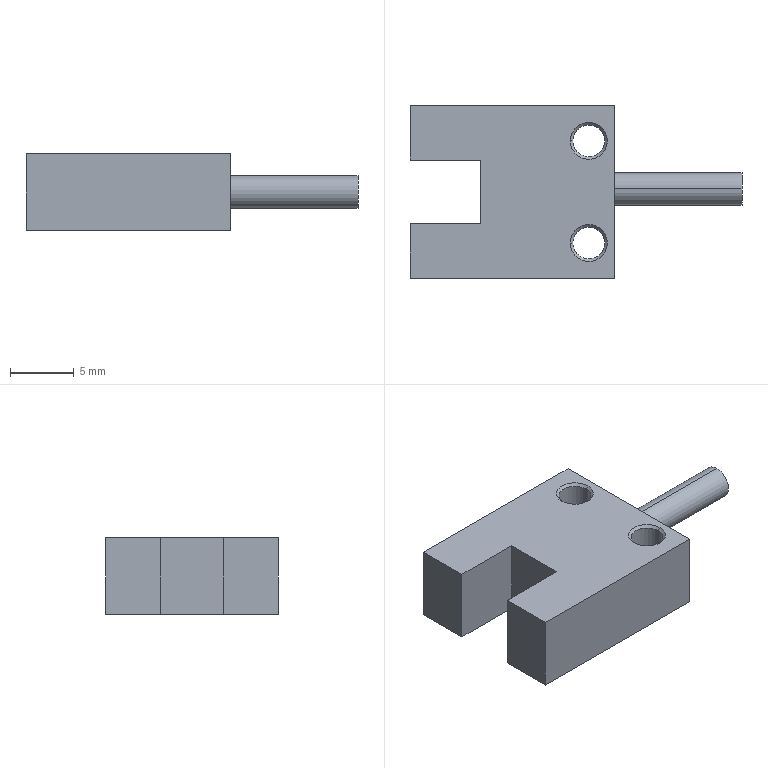Part | SolidWorks | features BaseBody 1 | 1 solid | 25 faces | box 26 x 13.5 x 6 mm | volume 1123 mm3 | plane 11 | cone 8 | cylinder 6 | commonest cylinder face diameters 2.5 x4 2.557 x2
STEP:
#1=CARTESIAN_POINT('',(4.191,-0.7465,0.2));
#2=VERTEX_POINT('',#1);
#3=CARTESIAN_POINT('',(1.691,-0.7465,0.2));
#4=VERTEX_POINT('',#3);
#5=CARTESIAN_POINT('',(2.941,-0.7465,0.2));
#6=DIRECTION('',(0.,0.,-1.));
#7=DIRECTION('',(-1.,0.,0.));
#8=AXIS2_PLACEMENT_3D('',#5,#6,#7);
#9=CIRCLE('',#8,1.25);
#10=EDGE_CURVE('',#2,#4,#9,.T.);
#11=ORIENTED_EDGE('',*,*,#10,.F.);
#12=CARTESIAN_POINT('',(4.391,-0.7465,0.));
#13=VERTEX_POINT('',#12);
#14=CARTESIAN_POINT('',(4.391,-0.7465,0.));
#15=DIRECTION('',(0.7071,0.,-0.7071));
#16=VECTOR('',#15,1000.);
#17=LINE('',#14,#16);
#18=EDGE_CURVE('',#2,#13,#17,.T.);
#19=ORIENTED_EDGE('',*,*,#18,.T.);
#20=CARTESIAN_POINT('',(1.491,-0.7465,0.));
#21=VERTEX_POINT('',#20);
#22=CARTESIAN_POINT('',(2.941,-0.7465,0.));
#23=DIRECTION('',(0.,0.,-1.));
#24=DIRECTION('',(-1.,0.,0.));
#25=AXIS2_PLACEMENT_3D('',#22,#23,#24);
#26=CIRCLE('',#25,1.45);
#27=EDGE_CURVE('',#13,#21,#26,.T.);
#28=ORIENTED_EDGE('',*,*,#27,.T.);
#29=CARTESIAN_POINT('',(1.491,-0.7465,0.));
#30=DIRECTION('',(-0.7071,0.,-0.7071));
#31=VECTOR('',#30,1000.);
#32=LINE('',#29,#31);
#33=EDGE_CURVE('',#4,#21,#32,.T.);
#34=ORIENTED_EDGE('',*,*,#33,.F.);
#35=EDGE_LOOP('',(#11,#19,#28,#34));
#36=FACE_OUTER_BOUND('',#35,.T.);
#37=CARTESIAN_POINT('',(2.941,-0.7465,0.));
#38=DIRECTION('',(0.,0.,-1.));
#39=DIRECTION('',(-1.,0.,0.));
#40=AXIS2_PLACEMENT_3D('',#37,#38,#39);
#41=CONICAL_SURFACE('',#40,1.45,0.7854);
#42=ADVANCED_FACE('',(#36),#41,.F.);
#43=CARTESIAN_POINT('',(4.191,7.253,0.2));
#44=VERTEX_POINT('',#43);
#45=CARTESIAN_POINT('',(1.691,7.253,0.2));
#46=VERTEX_POINT('',#45);
#47=CARTESIAN_POINT('',(2.941,7.253,0.2));
#48=DIRECTION('',(0.,0.,-1.));
#49=DIRECTION('',(-1.,0.,0.));
#50=AXIS2_PLACEMENT_3D('',#47,#48,#49);
#51=CIRCLE('',#50,1.25);
#52=EDGE_CURVE('',#44,#46,#51,.T.);
#53=ORIENTED_EDGE('',*,*,#52,.F.);
#54=CARTESIAN_POINT('',(4.391,7.253,0.));
#55=VERTEX_POINT('',#54);
#56=CARTESIAN_POINT('',(4.391,7.253,0.));
#57=DIRECTION('',(0.7071,0.,-0.7071));
#58=VECTOR('',#57,1000.);
#59=LINE('',#56,#58);
#60=EDGE_CURVE('',#44,#55,#59,.T.);
#61=ORIENTED_EDGE('',*,*,#60,.T.);
#62=CARTESIAN_POINT('',(1.491,7.253,0.));
#63=VERTEX_POINT('',#62);
#64=CARTESIAN_POINT('',(2.941,7.253,0.));
#65=DIRECTION('',(0.,0.,-1.));
#66=DIRECTION('',(-1.,0.,0.));
#67=AXIS2_PLACEMENT_3D('',#64,#65,#66);
#68=CIRCLE('',#67,1.45);
#69=EDGE_CURVE('',#55,#63,#68,.T.);
#70=ORIENTED_EDGE('',*,*,#69,.T.);
#71=CARTESIAN_POINT('',(1.491,7.253,0.));
#72=DIRECTION('',(-0.7071,0.,-0.7071));
#73=VECTOR('',#72,1000.);
#74=LINE('',#71,#73);
#75=EDGE_CURVE('',#46,#63,#74,.T.);
#76=ORIENTED_EDGE('',*,*,#75,.F.);
#77=EDGE_LOOP('',(#53,#61,#70,#76));
#78=FACE_OUTER_BOUND('',#77,.T.);
#79=CARTESIAN_POINT('',(2.941,7.253,0.));
#80=DIRECTION('',(0.,0.,-1.));
#81=DIRECTION('',(-1.,0.,0.));
#82=AXIS2_PLACEMENT_3D('',#79,#80,#81);
#83=CONICAL_SURFACE('',#82,1.45,0.7854);
#84=ADVANCED_FACE('',(#78),#83,.F.);
#85=CARTESIAN_POINT('',(4.191,-0.7465,5.8));
#86=VERTEX_POINT('',#85);
#87=CARTESIAN_POINT('',(1.691,-0.7465,5.8));
#88=VERTEX_POINT('',#87);
#89=CARTESIAN_POINT('',(2.941,-0.7465,5.8));
#90=DIRECTION('',(0.,0.,-1.));
#91=DIRECTION('',(-1.,0.,0.));
#92=AXIS2_PLACEMENT_3D('',#89,#90,#91);
#93=CIRCLE('',#92,1.25);
#94=EDGE_CURVE('',#86,#88,#93,.T.);
#95=ORIENTED_EDGE('',*,*,#94,.F.);
#96=CARTESIAN_POINT('',(4.191,-0.7465,6.));
#97=DIRECTION('',(0.,0.,-1.));
#98=VECTOR('',#97,1000.);
#99=LINE('',#96,#98);
#100=EDGE_CURVE('',#86,#2,#99,.T.);
#101=ORIENTED_EDGE('',*,*,#100,.T.);
#102=ORIENTED_EDGE('',*,*,#10,.T.);
#103=CARTESIAN_POINT('',(1.691,-0.7465,6.));
#104=DIRECTION('',(0.,0.,-1.));
#105=VECTOR('',#104,1000.);
#106=LINE('',#103,#105);
#107=EDGE_CURVE('',#88,#4,#106,.T.);
#108=ORIENTED_EDGE('',*,*,#107,.F.);
#109=EDGE_LOOP('',(#95,#101,#102,#108));
#110=FACE_OUTER_BOUND('',#109,.T.);
#111=CARTESIAN_POINT('',(2.941,-0.7465,6.));
#112=DIRECTION('',(0.,0.,-1.));
#113=DIRECTION('',(-1.,0.,0.));
#114=AXIS2_PLACEMENT_3D('',#111,#112,#113);
#115=CYLINDRICAL_SURFACE('',#114,1.25);
#116=ADVANCED_FACE('',(#110),#115,.F.);
#117=CARTESIAN_POINT('',(4.191,7.253,5.8));
#118=VERTEX_POINT('',#117);
#119=CARTESIAN_POINT('',(1.691,7.253,5.8));
#120=VERTEX_POINT('',#119);
#121=CARTESIAN_POINT('',(2.941,7.253,5.8));
#122=DIRECTION('',(0.,0.,-1.));
#123=DIRECTION('',(-1.,0.,0.));
#124=AXIS2_PLACEMENT_3D('',#121,#122,#123);
#125=CIRCLE('',#124,1.25);
#126=EDGE_CURVE('',#118,#120,#125,.T.);
#127=ORIENTED_EDGE('',*,*,#126,.F.);
#128=CARTESIAN_POINT('',(4.191,7.253,6.));
#129=DIRECTION('',(0.,0.,-1.));
#130=VECTOR('',#129,1000.);
#131=LINE('',#128,#130);
#132=EDGE_CURVE('',#118,#44,#131,.T.);
#133=ORIENTED_EDGE('',*,*,#132,.T.);
#134=ORIENTED_EDGE('',*,*,#52,.T.);
#135=CARTESIAN_POINT('',(1.691,7.253,6.));
#136=DIRECTION('',(0.,0.,-1.));
#137=VECTOR('',#136,1000.);
#138=LINE('',#135,#137);
#139=EDGE_CURVE('',#120,#46,#138,.T.);
#140=ORIENTED_EDGE('',*,*,#139,.F.);
#141=EDGE_LOOP('',(#127,#133,#134,#140));
#142=FACE_OUTER_BOUND('',#141,.T.);
#143=CARTESIAN_POINT('',(2.941,7.253,6.));
#144=DIRECTION('',(0.,0.,-1.));
#145=DIRECTION('',(-1.,0.,0.));
#146=AXIS2_PLACEMENT_3D('',#143,#144,#145);
#147=CYLINDRICAL_SURFACE('',#146,1.25);
#148=ADVANCED_FACE('',(#142),#147,.F.);
#149=CARTESIAN_POINT('',(4.941,3.503,4.278));
#150=VERTEX_POINT('',#149);
#151=CARTESIAN_POINT('',(4.941,3.503,1.722));
#152=VERTEX_POINT('',#151);
#153=CARTESIAN_POINT('',(4.941,3.503,3.));
#154=DIRECTION('',(-1.,0.,0.));
#155=DIRECTION('',(0.,0.,-1.));
#156=AXIS2_PLACEMENT_3D('',#153,#154,#155);
#157=CIRCLE('',#156,1.278);
#158=EDGE_CURVE('',#150,#152,#157,.T.);
#159=ORIENTED_EDGE('',*,*,#158,.F.);
#160=CARTESIAN_POINT('',(14.941,3.503,4.278));
#161=VERTEX_POINT('',#160);
#162=CARTESIAN_POINT('',(4.941,3.503,4.278));
#163=DIRECTION('',(1.,0.,0.));
#164=VECTOR('',#163,1000.);
#165=LINE('',#162,#164);
#166=EDGE_CURVE('',#150,#161,#165,.T.);
#167=ORIENTED_EDGE('',*,*,#166,.T.);
#168=CARTESIAN_POINT('',(14.941,3.503,1.722));
#169=VERTEX_POINT('',#168);
#170=CARTESIAN_POINT('',(14.941,3.503,3.));
#171=DIRECTION('',(-1.,0.,0.));
#172=DIRECTION('',(0.,0.,-1.));
#173=AXIS2_PLACEMENT_3D('',#170,#171,#172);
#174=CIRCLE('',#173,1.278);
#175=EDGE_CURVE('',#161,#169,#174,.T.);
#176=ORIENTED_EDGE('',*,*,#175,.T.);
#177=CARTESIAN_POINT('',(4.941,3.503,1.722));
#178=DIRECTION('',(1.,0.,0.));
#179=VECTOR('',#178,1000.);
#180=LINE('',#177,#179);
#181=EDGE_CURVE('',#152,#169,#180,.T.);
#182=ORIENTED_EDGE('',*,*,#181,.F.);
#183=EDGE_LOOP('',(#159,#167,#176,#182));
#184=FACE_OUTER_BOUND('',#183,.T.);
#185=CARTESIAN_POINT('',(4.941,3.503,3.));
#186=DIRECTION('',(1.,0.,0.));
#187=DIRECTION('',(0.,0.,-1.));
#188=AXIS2_PLACEMENT_3D('',#185,#186,#187);
#189=CYLINDRICAL_SURFACE('',#188,1.278);
#190=ADVANCED_FACE('',(#184),#189,.T.);
#191=ORIENTED_EDGE('',*,*,#94,.T.);
#192=CARTESIAN_POINT('',(1.491,-0.7465,6.));
#193=VERTEX_POINT('',#192);
#194=CARTESIAN_POINT('',(1.491,-0.7465,6.));
#195=DIRECTION('',(-0.7071,0.,0.7071));
#196=VECTOR('',#195,1000.);
#197=LINE('',#194,#196);
#198=EDGE_CURVE('',#88,#193,#197,.T.);
#199=ORIENTED_EDGE('',*,*,#198,.T.);
#200=CARTESIAN_POINT('',(4.391,-0.7465,6.));
#201=VERTEX_POINT('',#200);
#202=CARTESIAN_POINT('',(2.941,-0.7465,6.));
#203=DIRECTION('',(0.,0.,-1.));
#204=DIRECTION('',(1.,0.,0.));
#205=AXIS2_PLACEMENT_3D('',#202,#203,#204);
#206=CIRCLE('',#205,1.45);
#207=EDGE_CURVE('',#201,#193,#206,.T.);
#208=ORIENTED_EDGE('',*,*,#207,.F.);
#209=CARTESIAN_POINT('',(4.391,-0.7465,6.));
#210=DIRECTION('',(0.7071,0.,0.7071));
#211=VECTOR('',#210,1000.);
#212=LINE('',#209,#211);
#213=EDGE_CURVE('',#86,#201,#212,.T.);
#214=ORIENTED_EDGE('',*,*,#213,.F.);
#215=EDGE_LOOP('',(#191,#199,#208,#214));
#216=FACE_OUTER_BOUND('',#215,.T.);
#217=CARTESIAN_POINT('',(2.941,-0.7465,6.));
#218=DIRECTION('',(0.,0.,1.));
#219=DIRECTION('',(1.,0.,0.));
#220=AXIS2_PLACEMENT_3D('',#217,#218,#219);
#221=CONICAL_SURFACE('',#220,1.45,0.7854);
#222=ADVANCED_FACE('',(#216),#221,.F.);
#223=ORIENTED_EDGE('',*,*,#126,.T.);
#224=CARTESIAN_POINT('',(1.491,7.253,6.));
#225=VERTEX_POINT('',#224);
#226=CARTESIAN_POINT('',(1.491,7.253,6.));
#227=DIRECTION('',(-0.7071,0.,0.7071));
#228=VECTOR('',#227,1000.);
#229=LINE('',#226,#228);
#230=EDGE_CURVE('',#120,#225,#229,.T.);
#231=ORIENTED_EDGE('',*,*,#230,.T.);
#232=CARTESIAN_POINT('',(4.391,7.253,6.));
#233=VERTEX_POINT('',#232);
#234=CARTESIAN_POINT('',(2.941,7.253,6.));
#235=DIRECTION('',(0.,0.,-1.));
#236=DIRECTION('',(1.,0.,0.));
#237=AXIS2_PLACEMENT_3D('',#234,#235,#236);
#238=CIRCLE('',#237,1.45);
#239=EDGE_CURVE('',#233,#225,#238,.T.);
#240=ORIENTED_EDGE('',*,*,#239,.F.);
#241=CARTESIAN_POINT('',(4.391,7.253,6.));
#242=DIRECTION('',(0.7071,0.,0.7071));
#243=VECTOR('',#242,1000.);
#244=LINE('',#241,#243);
#245=EDGE_CURVE('',#118,#233,#244,.T.);
#246=ORIENTED_EDGE('',*,*,#245,.F.);
#247=EDGE_LOOP('',(#223,#231,#240,#246));
#248=FACE_OUTER_BOUND('',#247,.T.);
#249=CARTESIAN_POINT('',(2.941,7.253,6.));
#250=DIRECTION('',(0.,0.,1.));
#251=DIRECTION('',(1.,0.,0.));
#252=AXIS2_PLACEMENT_3D('',#249,#250,#251);
#253=CONICAL_SURFACE('',#252,1.45,0.7854);
#254=ADVANCED_FACE('',(#248),#253,.F.);
#255=CARTESIAN_POINT('',(2.941,-0.7465,0.));
#256=DIRECTION('',(0.,0.,-1.));
#257=DIRECTION('',(-1.,0.,0.));
#258=AXIS2_PLACEMENT_3D('',#255,#256,#257);
#259=CIRCLE('',#258,1.45);
#260=EDGE_CURVE('',#21,#13,#259,.T.);
#261=ORIENTED_EDGE('',*,*,#260,.F.);
#262=ORIENTED_EDGE('',*,*,#27,.F.);
#263=EDGE_LOOP('',(#261,#262));
#264=FACE_BOUND('',#263,.T.);
#265=CARTESIAN_POINT('',(2.941,7.253,0.));
#266=DIRECTION('',(0.,0.,-1.));
#267=DIRECTION('',(-1.,0.,0.));
#268=AXIS2_PLACEMENT_3D('',#265,#266,#267);
#269=CIRCLE('',#268,1.45);
#270=EDGE_CURVE('',#63,#55,#269,.T.);
#271=ORIENTED_EDGE('',*,*,#270,.F.);
#272=ORIENTED_EDGE('',*,*,#69,.F.);
#273=EDGE_LOOP('',(#271,#272));
#274=FACE_BOUND('',#273,.T.);
#275=CARTESIAN_POINT('',(-11.059,0.7535,0.));
#276=VERTEX_POINT('',#275);
#277=CARTESIAN_POINT('',(-11.059,-3.497,0.));
#278=VERTEX_POINT('',#277);
#279=CARTESIAN_POINT('',(-11.059,3.253,0.));
#280=DIRECTION('',(0.,-1.,0.));
#281=VECTOR('',#280,1000.);
#282=LINE('',#279,#281);
#283=EDGE_CURVE('',#276,#278,#282,.T.);
#284=ORIENTED_EDGE('',*,*,#283,.F.);
#285=CARTESIAN_POINT('',(-5.559,0.7535,0.));
#286=VERTEX_POINT('',#285);
#287=CARTESIAN_POINT('',(-3.491,0.7535,0.));
#288=DIRECTION('',(-1.,0.,0.));
#289=VECTOR('',#288,1000.);
#290=LINE('',#287,#289);
#291=EDGE_CURVE('',#286,#276,#290,.T.);
#292=ORIENTED_EDGE('',*,*,#291,.F.);
#293=CARTESIAN_POINT('',(-5.559,5.753,0.));
#294=VERTEX_POINT('',#293);
#295=CARTESIAN_POINT('',(-5.559,3.253,0.));
#296=DIRECTION('',(0.,-1.,0.));
#297=VECTOR('',#296,1000.);
#298=LINE('',#295,#297);
#299=EDGE_CURVE('',#294,#286,#298,.T.);
#300=ORIENTED_EDGE('',*,*,#299,.F.);
#301=CARTESIAN_POINT('',(-11.059,5.753,0.));
#302=VERTEX_POINT('',#301);
#303=CARTESIAN_POINT('',(-3.491,5.753,0.));
#304=DIRECTION('',(1.,0.,0.));
#305=VECTOR('',#304,1000.);
#306=LINE('',#303,#305);
#307=EDGE_CURVE('',#302,#294,#306,.T.);
#308=ORIENTED_EDGE('',*,*,#307,.F.);
#309=CARTESIAN_POINT('',(-11.059,10.003,0.));
#310=VERTEX_POINT('',#309);
#311=CARTESIAN_POINT('',(-11.059,3.253,0.));
#312=DIRECTION('',(0.,-1.,0.));
#313=VECTOR('',#312,1000.);
#314=LINE('',#311,#313);
#315=EDGE_CURVE('',#310,#302,#314,.T.);
#316=ORIENTED_EDGE('',*,*,#315,.F.);
#317=CARTESIAN_POINT('',(4.941,10.003,0.));
#318=VERTEX_POINT('',#317);
#319=CARTESIAN_POINT('',(-3.491,10.003,0.));
#320=DIRECTION('',(-1.,0.,0.));
#321=VECTOR('',#320,1000.);
#322=LINE('',#319,#321);
#323=EDGE_CURVE('',#318,#310,#322,.T.);
#324=ORIENTED_EDGE('',*,*,#323,.F.);
#325=CARTESIAN_POINT('',(4.941,-3.497,0.));
#326=VERTEX_POINT('',#325);
#327=CARTESIAN_POINT('',(4.941,3.253,0.));
#328=DIRECTION('',(0.,1.,0.));
#329=VECTOR('',#328,1000.);
#330=LINE('',#327,#329);
#331=EDGE_CURVE('',#326,#318,#330,.T.);
#332=ORIENTED_EDGE('',*,*,#331,.F.);
#333=CARTESIAN_POINT('',(-3.491,-3.497,0.));
#334=DIRECTION('',(1.,0.,0.));
#335=VECTOR('',#334,1000.);
#336=LINE('',#333,#335);
#337=EDGE_CURVE('',#278,#326,#336,.T.);
#338=ORIENTED_EDGE('',*,*,#337,.F.);
#339=EDGE_LOOP('',(#284,#292,#300,#308,#316,#324,#332,#338));
#340=FACE_OUTER_BOUND('',#339,.T.);
#341=CARTESIAN_POINT('',(-3.491,3.253,0.));
#342=DIRECTION('',(0.,0.,1.));
#343=DIRECTION('',(1.,0.,0.));
#344=AXIS2_PLACEMENT_3D('',#341,#342,#343);
#345=PLANE('',#344);
#346=ADVANCED_FACE('',(#264,#274,#340),#345,.F.);
#347=ORIENTED_EDGE('',*,*,#18,.F.);
#348=CARTESIAN_POINT('',(2.941,-0.7465,0.2));
#349=DIRECTION('',(0.,0.,-1.));
#350=DIRECTION('',(-1.,0.,0.));
#351=AXIS2_PLACEMENT_3D('',#348,#349,#350);
#352=CIRCLE('',#351,1.25);
#353=EDGE_CURVE('',#4,#2,#352,.T.);
#354=ORIENTED_EDGE('',*,*,#353,.F.);
#355=ORIENTED_EDGE('',*,*,#33,.T.);
#356=ORIENTED_EDGE('',*,*,#260,.T.);
#357=EDGE_LOOP('',(#347,#354,#355,#356));
#358=FACE_OUTER_BOUND('',#357,.T.);
#359=CARTESIAN_POINT('',(2.941,-0.7465,0.));
#360=DIRECTION('',(0.,0.,-1.));
#361=DIRECTION('',(-1.,0.,0.));
#362=AXIS2_PLACEMENT_3D('',#359,#360,#361);
#363=CONICAL_SURFACE('',#362,1.45,0.7854);
#364=ADVANCED_FACE('',(#358),#363,.F.);
#365=ORIENTED_EDGE('',*,*,#60,.F.);
#366=CARTESIAN_POINT('',(2.941,7.253,0.2));
#367=DIRECTION('',(0.,0.,-1.));
#368=DIRECTION('',(-1.,0.,0.));
#369=AXIS2_PLACEMENT_3D('',#366,#367,#368);
#370=CIRCLE('',#369,1.25);
#371=EDGE_CURVE('',#46,#44,#370,.T.);
#372=ORIENTED_EDGE('',*,*,#371,.F.);
#373=ORIENTED_EDGE('',*,*,#75,.T.);
#374=ORIENTED_EDGE('',*,*,#270,.T.);
#375=EDGE_LOOP('',(#365,#372,#373,#374));
#376=FACE_OUTER_BOUND('',#375,.T.);
#377=CARTESIAN_POINT('',(2.941,7.253,0.));
#378=DIRECTION('',(0.,0.,-1.));
#379=DIRECTION('',(-1.,0.,0.));
#380=AXIS2_PLACEMENT_3D('',#377,#378,#379);
#381=CONICAL_SURFACE('',#380,1.45,0.7854);
#382=ADVANCED_FACE('',(#376),#381,.F.);
#383=ORIENTED_EDGE('',*,*,#337,.T.);
#384=CARTESIAN_POINT('',(4.941,-3.497,6.));
#385=VERTEX_POINT('',#384);
#386=CARTESIAN_POINT('',(4.941,-3.497,0.));
#387=DIRECTION('',(0.,0.,1.));
#388=VECTOR('',#387,1000.);
#389=LINE('',#386,#388);
#390=EDGE_CURVE('',#326,#385,#389,.T.);
#391=ORIENTED_EDGE('',*,*,#390,.T.);
#392=CARTESIAN_POINT('',(-11.059,-3.497,6.));
#393=VERTEX_POINT('',#392);
#394=CARTESIAN_POINT('',(4.941,-3.497,6.));
#395=DIRECTION('',(-1.,0.,0.));
#396=VECTOR('',#395,1000.);
#397=LINE('',#394,#396);
#398=EDGE_CURVE('',#385,#393,#397,.T.);
#399=ORIENTED_EDGE('',*,*,#398,.T.);
#400=CARTESIAN_POINT('',(-11.059,-3.497,0.));
#401=DIRECTION('',(0.,0.,-1.));
#402=VECTOR('',#401,1000.);
#403=LINE('',#400,#402);
#404=EDGE_CURVE('',#393,#278,#403,.T.);
#405=ORIENTED_EDGE('',*,*,#404,.T.);
#406=EDGE_LOOP('',(#383,#391,#399,#405));
#407=FACE_OUTER_BOUND('',#406,.T.);
#408=CARTESIAN_POINT('',(4.941,-3.497,0.));
#409=DIRECTION('',(0.,-1.,0.));
#410=DIRECTION('',(0.,0.,-1.));
#411=AXIS2_PLACEMENT_3D('',#408,#409,#410);
#412=PLANE('',#411);
#413=ADVANCED_FACE('',(#407),#412,.T.);
#414=ORIENTED_EDGE('',*,*,#283,.T.);
#415=ORIENTED_EDGE('',*,*,#404,.F.);
#416=CARTESIAN_POINT('',(-11.059,0.7535,6.));
#417=VERTEX_POINT('',#416);
#418=CARTESIAN_POINT('',(-11.059,-3.497,6.));
#419=DIRECTION('',(0.,1.,0.));
#420=VECTOR('',#419,1000.);
#421=LINE('',#418,#420);
#422=EDGE_CURVE('',#393,#417,#421,.T.);
#423=ORIENTED_EDGE('',*,*,#422,.T.);
#424=CARTESIAN_POINT('',(-11.059,0.7535,0.));
#425=DIRECTION('',(0.,0.,-1.));
#426=VECTOR('',#425,1000.);
#427=LINE('',#424,#426);
#428=EDGE_CURVE('',#417,#276,#427,.T.);
#429=ORIENTED_EDGE('',*,*,#428,.T.);
#430=EDGE_LOOP('',(#414,#415,#423,#429));
#431=FACE_OUTER_BOUND('',#430,.T.);
#432=CARTESIAN_POINT('',(-11.059,-3.497,0.));
#433=DIRECTION('',(-1.,0.,0.));
#434=DIRECTION('',(0.,0.,1.));
#435=AXIS2_PLACEMENT_3D('',#432,#433,#434);
#436=PLANE('',#435);
#437=ADVANCED_FACE('',(#431),#436,.T.);
#438=ORIENTED_EDGE('',*,*,#291,.T.);
#439=ORIENTED_EDGE('',*,*,#428,.F.);
#440=CARTESIAN_POINT('',(-5.559,0.7535,6.));
#441=VERTEX_POINT('',#440);
#442=CARTESIAN_POINT('',(-11.059,0.7535,6.));
#443=DIRECTION('',(1.,0.,0.));
#444=VECTOR('',#443,1000.);
#445=LINE('',#442,#444);
#446=EDGE_CURVE('',#417,#441,#445,.T.);
#447=ORIENTED_EDGE('',*,*,#446,.T.);
#448=CARTESIAN_POINT('',(-5.559,0.7535,0.));
#449=DIRECTION('',(0.,0.,-1.));
#450=VECTOR('',#449,1000.);
#451=LINE('',#448,#450);
#452=EDGE_CURVE('',#441,#286,#451,.T.);
#453=ORIENTED_EDGE('',*,*,#452,.T.);
#454=EDGE_LOOP('',(#438,#439,#447,#453));
#455=FACE_OUTER_BOUND('',#454,.T.);
#456=CARTESIAN_POINT('',(-11.059,0.7535,0.));
#457=DIRECTION('',(0.,1.,0.));
#458=DIRECTION('',(0.,0.,1.));
#459=AXIS2_PLACEMENT_3D('',#456,#457,#458);
#460=PLANE('',#459);
#461=ADVANCED_FACE('',(#455),#460,.T.);
#462=ORIENTED_EDGE('',*,*,#299,.T.);
#463=ORIENTED_EDGE('',*,*,#452,.F.);
#464=CARTESIAN_POINT('',(-5.559,5.753,6.));
#465=VERTEX_POINT('',#464);
#466=CARTESIAN_POINT('',(-5.559,0.7535,6.));
#467=DIRECTION('',(0.,1.,0.));
#468=VECTOR('',#467,1000.);
#469=LINE('',#466,#468);
#470=EDGE_CURVE('',#441,#465,#469,.T.);
#471=ORIENTED_EDGE('',*,*,#470,.T.);
#472=CARTESIAN_POINT('',(-5.559,5.753,0.));
#473=DIRECTION('',(0.,0.,-1.));
#474=VECTOR('',#473,1000.);
#475=LINE('',#472,#474);
#476=EDGE_CURVE('',#465,#294,#475,.T.);
#477=ORIENTED_EDGE('',*,*,#476,.T.);
#478=EDGE_LOOP('',(#462,#463,#471,#477));
#479=FACE_OUTER_BOUND('',#478,.T.);
#480=CARTESIAN_POINT('',(-5.559,0.7535,0.));
#481=DIRECTION('',(-1.,0.,0.));
#482=DIRECTION('',(0.,0.,1.));
#483=AXIS2_PLACEMENT_3D('',#480,#481,#482);
#484=PLANE('',#483);
#485=ADVANCED_FACE('',(#479),#484,.T.);
#486=ORIENTED_EDGE('',*,*,#307,.T.);
#487=ORIENTED_EDGE('',*,*,#476,.F.);
#488=CARTESIAN_POINT('',(-11.059,5.753,6.));
#489=VERTEX_POINT('',#488);
#490=CARTESIAN_POINT('',(-5.559,5.753,6.));
#491=DIRECTION('',(-1.,0.,0.));
#492=VECTOR('',#491,1000.);
#493=LINE('',#490,#492);
#494=EDGE_CURVE('',#465,#489,#493,.T.);
#495=ORIENTED_EDGE('',*,*,#494,.T.);
#496=CARTESIAN_POINT('',(-11.059,5.753,0.));
#497=DIRECTION('',(0.,0.,-1.));
#498=VECTOR('',#497,1000.);
#499=LINE('',#496,#498);
#500=EDGE_CURVE('',#489,#302,#499,.T.);
#501=ORIENTED_EDGE('',*,*,#500,.T.);
#502=EDGE_LOOP('',(#486,#487,#495,#501));
#503=FACE_OUTER_BOUND('',#502,.T.);
#504=CARTESIAN_POINT('',(-5.559,5.753,0.));
#505=DIRECTION('',(0.,-1.,0.));
#506=DIRECTION('',(0.,0.,-1.));
#507=AXIS2_PLACEMENT_3D('',#504,#505,#506);
#508=PLANE('',#507);
#509=ADVANCED_FACE('',(#503),#508,.T.);
#510=ORIENTED_EDGE('',*,*,#315,.T.);
#511=ORIENTED_EDGE('',*,*,#500,.F.);
#512=CARTESIAN_POINT('',(-11.059,10.003,6.));
#513=VERTEX_POINT('',#512);
#514=CARTESIAN_POINT('',(-11.059,5.753,6.));
#515=DIRECTION('',(0.,1.,0.));
#516=VECTOR('',#515,1000.);
#517=LINE('',#514,#516);
#518=EDGE_CURVE('',#489,#513,#517,.T.);
#519=ORIENTED_EDGE('',*,*,#518,.T.);
#520=CARTESIAN_POINT('',(-11.059,10.003,0.));
#521=DIRECTION('',(0.,0.,-1.));
#522=VECTOR('',#521,1000.);
#523=LINE('',#520,#522);
#524=EDGE_CURVE('',#513,#310,#523,.T.);
#525=ORIENTED_EDGE('',*,*,#524,.T.);
#526=EDGE_LOOP('',(#510,#511,#519,#525));
#527=FACE_OUTER_BOUND('',#526,.T.);
#528=CARTESIAN_POINT('',(-11.059,5.753,0.));
#529=DIRECTION('',(-1.,0.,0.));
#530=DIRECTION('',(0.,0.,1.));
#531=AXIS2_PLACEMENT_3D('',#528,#529,#530);
#532=PLANE('',#531);
#533=ADVANCED_FACE('',(#527),#532,.T.);
#534=ORIENTED_EDGE('',*,*,#323,.T.);
#535=ORIENTED_EDGE('',*,*,#524,.F.);
#536=CARTESIAN_POINT('',(4.941,10.003,6.));
#537=VERTEX_POINT('',#536);
#538=CARTESIAN_POINT('',(-11.059,10.003,6.));
#539=DIRECTION('',(1.,0.,0.));
#540=VECTOR('',#539,1000.);
#541=LINE('',#538,#540);
#542=EDGE_CURVE('',#513,#537,#541,.T.);
#543=ORIENTED_EDGE('',*,*,#542,.T.);
#544=CARTESIAN_POINT('',(4.941,10.003,0.));
#545=DIRECTION('',(0.,0.,-1.));
#546=VECTOR('',#545,1000.);
#547=LINE('',#544,#546);
#548=EDGE_CURVE('',#537,#318,#547,.T.);
#549=ORIENTED_EDGE('',*,*,#548,.T.);
#550=EDGE_LOOP('',(#534,#535,#543,#549));
#551=FACE_OUTER_BOUND('',#550,.T.);
#552=CARTESIAN_POINT('',(-11.059,10.003,0.));
#553=DIRECTION('',(0.,1.,0.));
#554=DIRECTION('',(0.,0.,1.));
#555=AXIS2_PLACEMENT_3D('',#552,#553,#554);
#556=PLANE('',#555);
#557=ADVANCED_FACE('',(#551),#556,.T.);
#558=CARTESIAN_POINT('',(4.941,3.503,3.));
#559=DIRECTION('',(-1.,0.,0.));
#560=DIRECTION('',(0.,0.,-1.));
#561=AXIS2_PLACEMENT_3D('',#558,#559,#560);
#562=CIRCLE('',#561,1.278);
#563=EDGE_CURVE('',#152,#150,#562,.T.);
#564=ORIENTED_EDGE('',*,*,#563,.T.);
#565=ORIENTED_EDGE('',*,*,#158,.T.);
#566=EDGE_LOOP('',(#564,#565));
#567=FACE_BOUND('',#566,.T.);
#568=ORIENTED_EDGE('',*,*,#331,.T.);
#569=ORIENTED_EDGE('',*,*,#548,.F.);
#570=CARTESIAN_POINT('',(4.941,10.003,6.));
#571=DIRECTION('',(0.,-1.,0.));
#572=VECTOR('',#571,1000.);
#573=LINE('',#570,#572);
#574=EDGE_CURVE('',#537,#385,#573,.T.);
#575=ORIENTED_EDGE('',*,*,#574,.T.);
#576=ORIENTED_EDGE('',*,*,#390,.F.);
#577=EDGE_LOOP('',(#568,#569,#575,#576));
#578=FACE_OUTER_BOUND('',#577,.T.);
#579=CARTESIAN_POINT('',(4.941,10.003,0.));
#580=DIRECTION('',(1.,0.,0.));
#581=DIRECTION('',(0.,0.,-1.));
#582=AXIS2_PLACEMENT_3D('',#579,#580,#581);
#583=PLANE('',#582);
#584=ADVANCED_FACE('',(#567,#578),#583,.T.);
#585=ORIENTED_EDGE('',*,*,#100,.F.);
#586=CARTESIAN_POINT('',(2.941,-0.7465,5.8));
#587=DIRECTION('',(0.,0.,-1.));
#588=DIRECTION('',(-1.,0.,0.));
#589=AXIS2_PLACEMENT_3D('',#586,#587,#588);
#590=CIRCLE('',#589,1.25);
#591=EDGE_CURVE('',#88,#86,#590,.T.);
#592=ORIENTED_EDGE('',*,*,#591,.F.);
#593=ORIENTED_EDGE('',*,*,#107,.T.);
#594=ORIENTED_EDGE('',*,*,#353,.T.);
#595=EDGE_LOOP('',(#585,#592,#593,#594));
#596=FACE_OUTER_BOUND('',#595,.T.);
#597=CARTESIAN_POINT('',(2.941,-0.7465,6.));
#598=DIRECTION('',(0.,0.,-1.));
#599=DIRECTION('',(-1.,0.,0.));
#600=AXIS2_PLACEMENT_3D('',#597,#598,#599);
#601=CYLINDRICAL_SURFACE('',#600,1.25);
#602=ADVANCED_FACE('',(#596),#601,.F.);
#603=ORIENTED_EDGE('',*,*,#132,.F.);
#604=CARTESIAN_POINT('',(2.941,7.253,5.8));
#605=DIRECTION('',(0.,0.,-1.));
#606=DIRECTION('',(-1.,0.,0.));
#607=AXIS2_PLACEMENT_3D('',#604,#605,#606);
#608=CIRCLE('',#607,1.25);
#609=EDGE_CURVE('',#120,#118,#608,.T.);
#610=ORIENTED_EDGE('',*,*,#609,.F.);
#611=ORIENTED_EDGE('',*,*,#139,.T.);
#612=ORIENTED_EDGE('',*,*,#371,.T.);
#613=EDGE_LOOP('',(#603,#610,#611,#612));
#614=FACE_OUTER_BOUND('',#613,.T.);
#615=CARTESIAN_POINT('',(2.941,7.253,6.));
#616=DIRECTION('',(0.,0.,-1.));
#617=DIRECTION('',(-1.,0.,0.));
#618=AXIS2_PLACEMENT_3D('',#615,#616,#617);
#619=CYLINDRICAL_SURFACE('',#618,1.25);
#620=ADVANCED_FACE('',(#614),#619,.F.);
#621=ORIENTED_EDGE('',*,*,#207,.T.);
#622=CARTESIAN_POINT('',(2.941,-0.7465,6.));
#623=DIRECTION('',(0.,0.,-1.));
#624=DIRECTION('',(1.,0.,0.));
#625=AXIS2_PLACEMENT_3D('',#622,#623,#624);
#626=CIRCLE('',#625,1.45);
#627=EDGE_CURVE('',#193,#201,#626,.T.);
#628=ORIENTED_EDGE('',*,*,#627,.T.);
#629=EDGE_LOOP('',(#621,#628));
#630=FACE_BOUND('',#629,.T.);
#631=ORIENTED_EDGE('',*,*,#239,.T.);
#632=CARTESIAN_POINT('',(2.941,7.253,6.));
#633=DIRECTION('',(0.,0.,-1.));
#634=DIRECTION('',(1.,0.,0.));
#635=AXIS2_PLACEMENT_3D('',#632,#633,#634);
#636=CIRCLE('',#635,1.45);
#637=EDGE_CURVE('',#225,#233,#636,.T.);
#638=ORIENTED_EDGE('',*,*,#637,.T.);
#639=EDGE_LOOP('',(#631,#638));
#640=FACE_BOUND('',#639,.T.);
#641=ORIENTED_EDGE('',*,*,#470,.F.);
#642=ORIENTED_EDGE('',*,*,#446,.F.);
#643=ORIENTED_EDGE('',*,*,#422,.F.);
#644=ORIENTED_EDGE('',*,*,#398,.F.);
#645=ORIENTED_EDGE('',*,*,#574,.F.);
#646=ORIENTED_EDGE('',*,*,#542,.F.);
#647=ORIENTED_EDGE('',*,*,#518,.F.);
#648=ORIENTED_EDGE('',*,*,#494,.F.);
#649=EDGE_LOOP('',(#641,#642,#643,#644,#645,#646,#647,#648));
#650=FACE_OUTER_BOUND('',#649,.T.);
#651=CARTESIAN_POINT('',(-3.491,3.253,6.));
#652=DIRECTION('',(0.,0.,1.));
#653=DIRECTION('',(1.,0.,0.));
#654=AXIS2_PLACEMENT_3D('',#651,#652,#653);
#655=PLANE('',#654);
#656=ADVANCED_FACE('',(#630,#640,#650),#655,.T.);
#657=ORIENTED_EDGE('',*,*,#166,.F.);
#658=ORIENTED_EDGE('',*,*,#563,.F.);
#659=ORIENTED_EDGE('',*,*,#181,.T.);
#660=CARTESIAN_POINT('',(14.941,3.503,3.));
#661=DIRECTION('',(-1.,0.,0.));
#662=DIRECTION('',(0.,0.,-1.));
#663=AXIS2_PLACEMENT_3D('',#660,#661,#662);
#664=CIRCLE('',#663,1.278);
#665=EDGE_CURVE('',#169,#161,#664,.T.);
#666=ORIENTED_EDGE('',*,*,#665,.T.);
#667=EDGE_LOOP('',(#657,#658,#659,#666));
#668=FACE_OUTER_BOUND('',#667,.T.);
#669=CARTESIAN_POINT('',(4.941,3.503,3.));
#670=DIRECTION('',(1.,0.,0.));
#671=DIRECTION('',(0.,0.,-1.));
#672=AXIS2_PLACEMENT_3D('',#669,#670,#671);
#673=CYLINDRICAL_SURFACE('',#672,1.278);
#674=ADVANCED_FACE('',(#668),#673,.T.);
#675=ORIENTED_EDGE('',*,*,#198,.F.);
#676=ORIENTED_EDGE('',*,*,#591,.T.);
#677=ORIENTED_EDGE('',*,*,#213,.T.);
#678=ORIENTED_EDGE('',*,*,#627,.F.);
#679=EDGE_LOOP('',(#675,#676,#677,#678));
#680=FACE_OUTER_BOUND('',#679,.T.);
#681=CARTESIAN_POINT('',(2.941,-0.7465,6.));
#682=DIRECTION('',(0.,0.,1.));
#683=DIRECTION('',(1.,0.,0.));
#684=AXIS2_PLACEMENT_3D('',#681,#682,#683);
#685=CONICAL_SURFACE('',#684,1.45,0.7854);
#686=ADVANCED_FACE('',(#680),#685,.F.);
#687=ORIENTED_EDGE('',*,*,#230,.F.);
#688=ORIENTED_EDGE('',*,*,#609,.T.);
#689=ORIENTED_EDGE('',*,*,#245,.T.);
#690=ORIENTED_EDGE('',*,*,#637,.F.);
#691=EDGE_LOOP('',(#687,#688,#689,#690));
#692=FACE_OUTER_BOUND('',#691,.T.);
#693=CARTESIAN_POINT('',(2.941,7.253,6.));
#694=DIRECTION('',(0.,0.,1.));
#695=DIRECTION('',(1.,0.,0.));
#696=AXIS2_PLACEMENT_3D('',#693,#694,#695);
#697=CONICAL_SURFACE('',#696,1.45,0.7854);
#698=ADVANCED_FACE('',(#692),#697,.F.);
#699=ORIENTED_EDGE('',*,*,#665,.F.);
#700=ORIENTED_EDGE('',*,*,#175,.F.);
#701=EDGE_LOOP('',(#699,#700));
#702=FACE_OUTER_BOUND('',#701,.T.);
#703=CARTESIAN_POINT('',(14.941,3.503,3.));
#704=DIRECTION('',(-1.,0.,0.));
#705=DIRECTION('',(0.,0.,1.));
#706=AXIS2_PLACEMENT_3D('',#703,#704,#705);
#707=PLANE('',#706);
#708=ADVANCED_FACE('',(#702),#707,.F.);
#709=CLOSED_SHELL('',(#42,#84,#116,#148,#190,#222,#254,#346,#364,#382,#413,#437,#461,#485,#509,#533,#557,#584,#602,#620,#656,#674,#686,#698,#708));
#710=MANIFOLD_SOLID_BREP('',#709);
#711=CARTESIAN_POINT('',(0.,0.,0.));
#712=DIRECTION('',(0.,0.,1.));
#713=DIRECTION('',(1.,0.,0.));
#714=AXIS2_PLACEMENT_3D('',#711,#712,#713);
#715=(LENGTH_UNIT()NAMED_UNIT(*)SI_UNIT(.MILLI.,.METRE.));
#716=UNCERTAINTY_MEASURE_WITH_UNIT(LENGTH_MEASURE(0.00001),#715,'','');
#717=(NAMED_UNIT(*)PLANE_ANGLE_UNIT()SI_UNIT($,.RADIAN.));
#718=(NAMED_UNIT(*)SI_UNIT($,.STERADIAN.)SOLID_ANGLE_UNIT());
#719=(GEOMETRIC_REPRESENTATION_CONTEXT(3)GLOBAL_UNCERTAINTY_ASSIGNED_CONTEXT((#716))GLOBAL_UNIT_ASSIGNED_CONTEXT((#715,#717,#718))REPRESENTATION_CONTEXT('',''));
#720=ADVANCED_BREP_SHAPE_REPRESENTATION('',(#710,#714),#719);